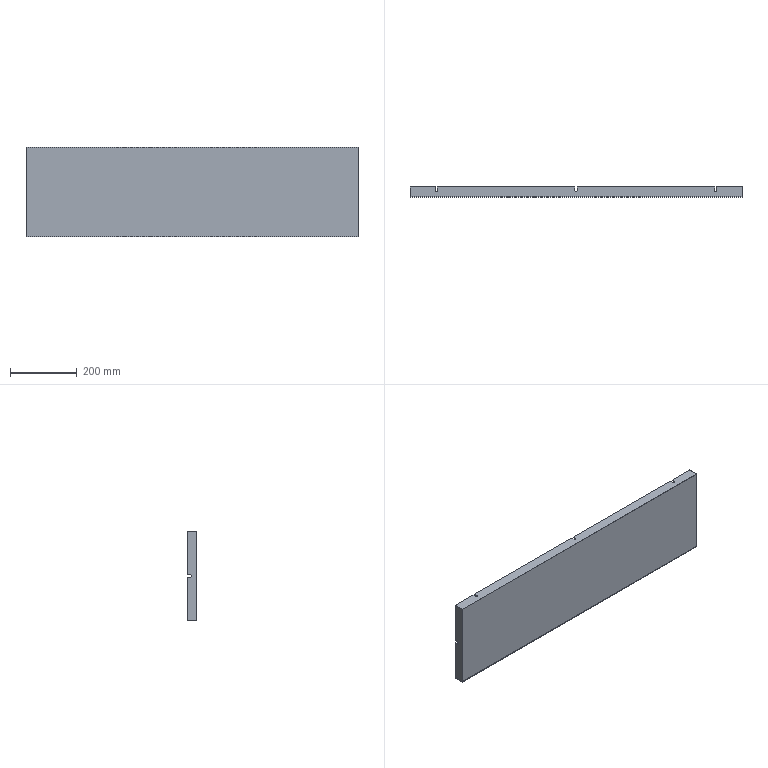Part | SolidWorks | features BaseBody 1 | 1 solid | 42 faces | box 998 x 30 x 268 mm | volume 508112 mm3 | plane 34 | cylinder 8 | commonest cylinder face diameters 7 x8
STEP:
#1=CARTESIAN_POINT('',(-416.5,20.,-132.5));
#2=VERTEX_POINT('',#1);
#3=CARTESIAN_POINT('',(-416.5,30.,-132.5));
#4=VERTEX_POINT('',#3);
#5=CARTESIAN_POINT('',(-416.5,30.,-132.5));
#6=DIRECTION('',(0.,1.,0.));
#7=VECTOR('',#6,1000.);
#8=LINE('',#5,#7);
#9=EDGE_CURVE('',#2,#4,#8,.T.);
#10=ORIENTED_EDGE('',*,*,#9,.T.);
#11=CARTESIAN_POINT('',(-416.5,30.,-134.));
#12=VERTEX_POINT('',#11);
#13=CARTESIAN_POINT('',(-416.5,30.,134.));
#14=DIRECTION('',(0.,0.,-1.));
#15=VECTOR('',#14,1000.);
#16=LINE('',#13,#15);
#17=EDGE_CURVE('',#4,#12,#16,.T.);
#18=ORIENTED_EDGE('',*,*,#17,.T.);
#19=CARTESIAN_POINT('',(-416.5,20.,-134.));
#20=VERTEX_POINT('',#19);
#21=CARTESIAN_POINT('',(-416.5,30.,-134.));
#22=DIRECTION('',(0.,-1.,0.));
#23=VECTOR('',#22,1000.);
#24=LINE('',#21,#23);
#25=EDGE_CURVE('',#12,#20,#24,.T.);
#26=ORIENTED_EDGE('',*,*,#25,.T.);
#27=CARTESIAN_POINT('',(-416.5,20.,134.));
#28=DIRECTION('',(0.,0.,-1.));
#29=VECTOR('',#28,1000.);
#30=LINE('',#27,#29);
#31=EDGE_CURVE('',#2,#20,#30,.T.);
#32=ORIENTED_EDGE('',*,*,#31,.F.);
#33=EDGE_LOOP('',(#10,#18,#26,#32));
#34=FACE_OUTER_BOUND('',#33,.T.);
#35=CARTESIAN_POINT('',(-416.5,30.,134.));
#36=DIRECTION('',(1.,0.,0.));
#37=DIRECTION('',(0.,1.,0.));
#38=AXIS2_PLACEMENT_3D('',#35,#36,#37);
#39=PLANE('',#38);
#40=ADVANCED_FACE('',(#34),#39,.F.);
#41=CARTESIAN_POINT('',(-423.5,20.,-132.5));
#42=VERTEX_POINT('',#41);
#43=CARTESIAN_POINT('',(-420.,20.,-132.5));
#44=DIRECTION('',(0.,0.,1.));
#45=DIRECTION('',(1.,0.,0.));
#46=AXIS2_PLACEMENT_3D('',#43,#44,#45);
#47=CIRCLE('',#46,3.5);
#48=EDGE_CURVE('',#42,#2,#47,.T.);
#49=ORIENTED_EDGE('',*,*,#48,.T.);
#50=ORIENTED_EDGE('',*,*,#31,.T.);
#51=CARTESIAN_POINT('',(-423.5,20.,-134.));
#52=VERTEX_POINT('',#51);
#53=CARTESIAN_POINT('',(-420.,20.,-134.));
#54=DIRECTION('',(0.,0.,-1.));
#55=DIRECTION('',(-1.,0.,0.));
#56=AXIS2_PLACEMENT_3D('',#53,#54,#55);
#57=CIRCLE('',#56,3.5);
#58=EDGE_CURVE('',#20,#52,#57,.T.);
#59=ORIENTED_EDGE('',*,*,#58,.T.);
#60=CARTESIAN_POINT('',(-423.5,20.,134.));
#61=DIRECTION('',(0.,0.,-1.));
#62=VECTOR('',#61,1000.);
#63=LINE('',#60,#62);
#64=EDGE_CURVE('',#42,#52,#63,.T.);
#65=ORIENTED_EDGE('',*,*,#64,.F.);
#66=EDGE_LOOP('',(#49,#50,#59,#65));
#67=FACE_OUTER_BOUND('',#66,.T.);
#68=CARTESIAN_POINT('',(-420.,20.,134.));
#69=DIRECTION('',(0.,0.,-1.));
#70=DIRECTION('',(-1.,0.,0.));
#71=AXIS2_PLACEMENT_3D('',#68,#69,#70);
#72=CYLINDRICAL_SURFACE('',#71,3.5);
#73=ADVANCED_FACE('',(#67),#72,.F.);
#74=CARTESIAN_POINT('',(-423.5,30.,-132.5));
#75=VERTEX_POINT('',#74);
#76=CARTESIAN_POINT('',(-423.5,30.,-132.5));
#77=DIRECTION('',(0.,-1.,0.));
#78=VECTOR('',#77,1000.);
#79=LINE('',#76,#78);
#80=EDGE_CURVE('',#75,#42,#79,.T.);
#81=ORIENTED_EDGE('',*,*,#80,.T.);
#82=ORIENTED_EDGE('',*,*,#64,.T.);
#83=CARTESIAN_POINT('',(-423.5,30.,-134.));
#84=VERTEX_POINT('',#83);
#85=CARTESIAN_POINT('',(-423.5,30.,-134.));
#86=DIRECTION('',(0.,1.,0.));
#87=VECTOR('',#86,1000.);
#88=LINE('',#85,#87);
#89=EDGE_CURVE('',#52,#84,#88,.T.);
#90=ORIENTED_EDGE('',*,*,#89,.T.);
#91=CARTESIAN_POINT('',(-423.5,30.,134.));
#92=DIRECTION('',(0.,0.,-1.));
#93=VECTOR('',#92,1000.);
#94=LINE('',#91,#93);
#95=EDGE_CURVE('',#75,#84,#94,.T.);
#96=ORIENTED_EDGE('',*,*,#95,.F.);
#97=EDGE_LOOP('',(#81,#82,#90,#96));
#98=FACE_OUTER_BOUND('',#97,.T.);
#99=CARTESIAN_POINT('',(-423.5,30.,134.));
#100=DIRECTION('',(-1.,0.,0.));
#101=DIRECTION('',(0.,0.,1.));
#102=AXIS2_PLACEMENT_3D('',#99,#100,#101);
#103=PLANE('',#102);
#104=ADVANCED_FACE('',(#98),#103,.F.);
#105=CARTESIAN_POINT('',(-423.5,20.,132.5));
#106=VERTEX_POINT('',#105);
#107=CARTESIAN_POINT('',(-423.5,30.,132.5));
#108=VERTEX_POINT('',#107);
#109=CARTESIAN_POINT('',(-423.5,30.,132.5));
#110=DIRECTION('',(0.,1.,0.));
#111=VECTOR('',#110,1000.);
#112=LINE('',#109,#111);
#113=EDGE_CURVE('',#106,#108,#112,.T.);
#114=ORIENTED_EDGE('',*,*,#113,.T.);
#115=CARTESIAN_POINT('',(-423.5,30.,134.));
#116=VERTEX_POINT('',#115);
#117=CARTESIAN_POINT('',(-423.5,30.,134.));
#118=DIRECTION('',(0.,0.,-1.));
#119=VECTOR('',#118,1000.);
#120=LINE('',#117,#119);
#121=EDGE_CURVE('',#116,#108,#120,.T.);
#122=ORIENTED_EDGE('',*,*,#121,.F.);
#123=CARTESIAN_POINT('',(-423.5,20.,134.));
#124=VERTEX_POINT('',#123);
#125=CARTESIAN_POINT('',(-423.5,30.,134.));
#126=DIRECTION('',(0.,1.,0.));
#127=VECTOR('',#126,1000.);
#128=LINE('',#125,#127);
#129=EDGE_CURVE('',#124,#116,#128,.T.);
#130=ORIENTED_EDGE('',*,*,#129,.F.);
#131=CARTESIAN_POINT('',(-423.5,20.,134.));
#132=DIRECTION('',(0.,0.,-1.));
#133=VECTOR('',#132,1000.);
#134=LINE('',#131,#133);
#135=EDGE_CURVE('',#124,#106,#134,.T.);
#136=ORIENTED_EDGE('',*,*,#135,.T.);
#137=EDGE_LOOP('',(#114,#122,#130,#136));
#138=FACE_OUTER_BOUND('',#137,.T.);
#139=CARTESIAN_POINT('',(-423.5,30.,134.));
#140=DIRECTION('',(-1.,0.,0.));
#141=DIRECTION('',(0.,0.,1.));
#142=AXIS2_PLACEMENT_3D('',#139,#140,#141);
#143=PLANE('',#142);
#144=ADVANCED_FACE('',(#138),#143,.F.);
#145=CARTESIAN_POINT('',(-416.5,20.,132.5));
#146=VERTEX_POINT('',#145);
#147=CARTESIAN_POINT('',(-420.,20.,132.5));
#148=DIRECTION('',(0.,0.,-1.));
#149=DIRECTION('',(-1.,0.,0.));
#150=AXIS2_PLACEMENT_3D('',#147,#148,#149);
#151=CIRCLE('',#150,3.5);
#152=EDGE_CURVE('',#146,#106,#151,.T.);
#153=ORIENTED_EDGE('',*,*,#152,.T.);
#154=ORIENTED_EDGE('',*,*,#135,.F.);
#155=CARTESIAN_POINT('',(-416.5,20.,134.));
#156=VERTEX_POINT('',#155);
#157=CARTESIAN_POINT('',(-420.,20.,134.));
#158=DIRECTION('',(0.,0.,-1.));
#159=DIRECTION('',(-1.,0.,0.));
#160=AXIS2_PLACEMENT_3D('',#157,#158,#159);
#161=CIRCLE('',#160,3.5);
#162=EDGE_CURVE('',#156,#124,#161,.T.);
#163=ORIENTED_EDGE('',*,*,#162,.F.);
#164=CARTESIAN_POINT('',(-416.5,20.,134.));
#165=DIRECTION('',(0.,0.,-1.));
#166=VECTOR('',#165,1000.);
#167=LINE('',#164,#166);
#168=EDGE_CURVE('',#156,#146,#167,.T.);
#169=ORIENTED_EDGE('',*,*,#168,.T.);
#170=EDGE_LOOP('',(#153,#154,#163,#169));
#171=FACE_OUTER_BOUND('',#170,.T.);
#172=CARTESIAN_POINT('',(-420.,20.,134.));
#173=DIRECTION('',(0.,0.,-1.));
#174=DIRECTION('',(-1.,0.,0.));
#175=AXIS2_PLACEMENT_3D('',#172,#173,#174);
#176=CYLINDRICAL_SURFACE('',#175,3.5);
#177=ADVANCED_FACE('',(#171),#176,.F.);
#178=CARTESIAN_POINT('',(-416.5,30.,132.5));
#179=VERTEX_POINT('',#178);
#180=CARTESIAN_POINT('',(-416.5,30.,132.5));
#181=DIRECTION('',(0.,-1.,0.));
#182=VECTOR('',#181,1000.);
#183=LINE('',#180,#182);
#184=EDGE_CURVE('',#179,#146,#183,.T.);
#185=ORIENTED_EDGE('',*,*,#184,.T.);
#186=ORIENTED_EDGE('',*,*,#168,.F.);
#187=CARTESIAN_POINT('',(-416.5,30.,134.));
#188=VERTEX_POINT('',#187);
#189=CARTESIAN_POINT('',(-416.5,30.,134.));
#190=DIRECTION('',(0.,-1.,0.));
#191=VECTOR('',#190,1000.);
#192=LINE('',#189,#191);
#193=EDGE_CURVE('',#188,#156,#192,.T.);
#194=ORIENTED_EDGE('',*,*,#193,.F.);
#195=CARTESIAN_POINT('',(-416.5,30.,134.));
#196=DIRECTION('',(0.,0.,-1.));
#197=VECTOR('',#196,1000.);
#198=LINE('',#195,#197);
#199=EDGE_CURVE('',#188,#179,#198,.T.);
#200=ORIENTED_EDGE('',*,*,#199,.T.);
#201=EDGE_LOOP('',(#185,#186,#194,#200));
#202=FACE_OUTER_BOUND('',#201,.T.);
#203=CARTESIAN_POINT('',(-416.5,30.,134.));
#204=DIRECTION('',(1.,0.,0.));
#205=DIRECTION('',(0.,1.,0.));
#206=AXIS2_PLACEMENT_3D('',#203,#204,#205);
#207=PLANE('',#206);
#208=ADVANCED_FACE('',(#202),#207,.F.);
#209=CARTESIAN_POINT('',(3.5,20.,-132.5));
#210=VERTEX_POINT('',#209);
#211=CARTESIAN_POINT('',(3.5,30.,-132.5));
#212=VERTEX_POINT('',#211);
#213=CARTESIAN_POINT('',(3.5,30.,-132.5));
#214=DIRECTION('',(0.,1.,0.));
#215=VECTOR('',#214,1000.);
#216=LINE('',#213,#215);
#217=EDGE_CURVE('',#210,#212,#216,.T.);
#218=ORIENTED_EDGE('',*,*,#217,.T.);
#219=CARTESIAN_POINT('',(3.5,30.,-134.));
#220=VERTEX_POINT('',#219);
#221=CARTESIAN_POINT('',(3.5,30.,134.));
#222=DIRECTION('',(0.,0.,-1.));
#223=VECTOR('',#222,1000.);
#224=LINE('',#221,#223);
#225=EDGE_CURVE('',#212,#220,#224,.T.);
#226=ORIENTED_EDGE('',*,*,#225,.T.);
#227=CARTESIAN_POINT('',(3.5,20.,-134.));
#228=VERTEX_POINT('',#227);
#229=CARTESIAN_POINT('',(3.5,30.,-134.));
#230=DIRECTION('',(0.,-1.,0.));
#231=VECTOR('',#230,1000.);
#232=LINE('',#229,#231);
#233=EDGE_CURVE('',#220,#228,#232,.T.);
#234=ORIENTED_EDGE('',*,*,#233,.T.);
#235=CARTESIAN_POINT('',(3.5,20.,134.));
#236=DIRECTION('',(0.,0.,-1.));
#237=VECTOR('',#236,1000.);
#238=LINE('',#235,#237);
#239=EDGE_CURVE('',#210,#228,#238,.T.);
#240=ORIENTED_EDGE('',*,*,#239,.F.);
#241=EDGE_LOOP('',(#218,#226,#234,#240));
#242=FACE_OUTER_BOUND('',#241,.T.);
#243=CARTESIAN_POINT('',(3.5,30.,134.));
#244=DIRECTION('',(1.,0.,0.));
#245=DIRECTION('',(0.,1.,0.));
#246=AXIS2_PLACEMENT_3D('',#243,#244,#245);
#247=PLANE('',#246);
#248=ADVANCED_FACE('',(#242),#247,.F.);
#249=CARTESIAN_POINT('',(-3.5,20.,-132.5));
#250=VERTEX_POINT('',#249);
#251=CARTESIAN_POINT('',(0.,20.,-132.5));
#252=DIRECTION('',(0.,0.,1.));
#253=DIRECTION('',(1.,0.,0.));
#254=AXIS2_PLACEMENT_3D('',#251,#252,#253);
#255=CIRCLE('',#254,3.5);
#256=EDGE_CURVE('',#250,#210,#255,.T.);
#257=ORIENTED_EDGE('',*,*,#256,.T.);
#258=ORIENTED_EDGE('',*,*,#239,.T.);
#259=CARTESIAN_POINT('',(-3.5,20.,-134.));
#260=VERTEX_POINT('',#259);
#261=CARTESIAN_POINT('',(0.,20.,-134.));
#262=DIRECTION('',(0.,0.,-1.));
#263=DIRECTION('',(-1.,0.,0.));
#264=AXIS2_PLACEMENT_3D('',#261,#262,#263);
#265=CIRCLE('',#264,3.5);
#266=EDGE_CURVE('',#228,#260,#265,.T.);
#267=ORIENTED_EDGE('',*,*,#266,.T.);
#268=CARTESIAN_POINT('',(-3.5,20.,134.));
#269=DIRECTION('',(0.,0.,-1.));
#270=VECTOR('',#269,1000.);
#271=LINE('',#268,#270);
#272=EDGE_CURVE('',#250,#260,#271,.T.);
#273=ORIENTED_EDGE('',*,*,#272,.F.);
#274=EDGE_LOOP('',(#257,#258,#267,#273));
#275=FACE_OUTER_BOUND('',#274,.T.);
#276=CARTESIAN_POINT('',(0.,20.,134.));
#277=DIRECTION('',(0.,0.,-1.));
#278=DIRECTION('',(-1.,0.,0.));
#279=AXIS2_PLACEMENT_3D('',#276,#277,#278);
#280=CYLINDRICAL_SURFACE('',#279,3.5);
#281=ADVANCED_FACE('',(#275),#280,.F.);
#282=CARTESIAN_POINT('',(-3.5,30.,-132.5));
#283=VERTEX_POINT('',#282);
#284=CARTESIAN_POINT('',(-3.5,30.,-132.5));
#285=DIRECTION('',(0.,-1.,0.));
#286=VECTOR('',#285,1000.);
#287=LINE('',#284,#286);
#288=EDGE_CURVE('',#283,#250,#287,.T.);
#289=ORIENTED_EDGE('',*,*,#288,.T.);
#290=ORIENTED_EDGE('',*,*,#272,.T.);
#291=CARTESIAN_POINT('',(-3.5,30.,-134.));
#292=VERTEX_POINT('',#291);
#293=CARTESIAN_POINT('',(-3.5,30.,-134.));
#294=DIRECTION('',(0.,1.,0.));
#295=VECTOR('',#294,1000.);
#296=LINE('',#293,#295);
#297=EDGE_CURVE('',#260,#292,#296,.T.);
#298=ORIENTED_EDGE('',*,*,#297,.T.);
#299=CARTESIAN_POINT('',(-3.5,30.,134.));
#300=DIRECTION('',(0.,0.,-1.));
#301=VECTOR('',#300,1000.);
#302=LINE('',#299,#301);
#303=EDGE_CURVE('',#283,#292,#302,.T.);
#304=ORIENTED_EDGE('',*,*,#303,.F.);
#305=EDGE_LOOP('',(#289,#290,#298,#304));
#306=FACE_OUTER_BOUND('',#305,.T.);
#307=CARTESIAN_POINT('',(-3.5,30.,134.));
#308=DIRECTION('',(-1.,0.,0.));
#309=DIRECTION('',(0.,0.,1.));
#310=AXIS2_PLACEMENT_3D('',#307,#308,#309);
#311=PLANE('',#310);
#312=ADVANCED_FACE('',(#306),#311,.F.);
#313=CARTESIAN_POINT('',(-3.5,20.,132.5));
#314=VERTEX_POINT('',#313);
#315=CARTESIAN_POINT('',(-3.5,30.,132.5));
#316=VERTEX_POINT('',#315);
#317=CARTESIAN_POINT('',(-3.5,30.,132.5));
#318=DIRECTION('',(0.,1.,0.));
#319=VECTOR('',#318,1000.);
#320=LINE('',#317,#319);
#321=EDGE_CURVE('',#314,#316,#320,.T.);
#322=ORIENTED_EDGE('',*,*,#321,.T.);
#323=CARTESIAN_POINT('',(-3.5,30.,134.));
#324=VERTEX_POINT('',#323);
#325=CARTESIAN_POINT('',(-3.5,30.,134.));
#326=DIRECTION('',(0.,0.,-1.));
#327=VECTOR('',#326,1000.);
#328=LINE('',#325,#327);
#329=EDGE_CURVE('',#324,#316,#328,.T.);
#330=ORIENTED_EDGE('',*,*,#329,.F.);
#331=CARTESIAN_POINT('',(-3.5,20.,134.));
#332=VERTEX_POINT('',#331);
#333=CARTESIAN_POINT('',(-3.5,30.,134.));
#334=DIRECTION('',(0.,1.,0.));
#335=VECTOR('',#334,1000.);
#336=LINE('',#333,#335);
#337=EDGE_CURVE('',#332,#324,#336,.T.);
#338=ORIENTED_EDGE('',*,*,#337,.F.);
#339=CARTESIAN_POINT('',(-3.5,20.,134.));
#340=DIRECTION('',(0.,0.,-1.));
#341=VECTOR('',#340,1000.);
#342=LINE('',#339,#341);
#343=EDGE_CURVE('',#332,#314,#342,.T.);
#344=ORIENTED_EDGE('',*,*,#343,.T.);
#345=EDGE_LOOP('',(#322,#330,#338,#344));
#346=FACE_OUTER_BOUND('',#345,.T.);
#347=CARTESIAN_POINT('',(-3.5,30.,134.));
#348=DIRECTION('',(-1.,0.,0.));
#349=DIRECTION('',(0.,0.,1.));
#350=AXIS2_PLACEMENT_3D('',#347,#348,#349);
#351=PLANE('',#350);
#352=ADVANCED_FACE('',(#346),#351,.F.);
#353=CARTESIAN_POINT('',(3.5,20.,132.5));
#354=VERTEX_POINT('',#353);
#355=CARTESIAN_POINT('',(0.,20.,132.5));
#356=DIRECTION('',(0.,0.,-1.));
#357=DIRECTION('',(-1.,0.,0.));
#358=AXIS2_PLACEMENT_3D('',#355,#356,#357);
#359=CIRCLE('',#358,3.5);
#360=EDGE_CURVE('',#354,#314,#359,.T.);
#361=ORIENTED_EDGE('',*,*,#360,.T.);
#362=ORIENTED_EDGE('',*,*,#343,.F.);
#363=CARTESIAN_POINT('',(3.5,20.,134.));
#364=VERTEX_POINT('',#363);
#365=CARTESIAN_POINT('',(0.,20.,134.));
#366=DIRECTION('',(0.,0.,-1.));
#367=DIRECTION('',(-1.,0.,0.));
#368=AXIS2_PLACEMENT_3D('',#365,#366,#367);
#369=CIRCLE('',#368,3.5);
#370=EDGE_CURVE('',#364,#332,#369,.T.);
#371=ORIENTED_EDGE('',*,*,#370,.F.);
#372=CARTESIAN_POINT('',(3.5,20.,134.));
#373=DIRECTION('',(0.,0.,-1.));
#374=VECTOR('',#373,1000.);
#375=LINE('',#372,#374);
#376=EDGE_CURVE('',#364,#354,#375,.T.);
#377=ORIENTED_EDGE('',*,*,#376,.T.);
#378=EDGE_LOOP('',(#361,#362,#371,#377));
#379=FACE_OUTER_BOUND('',#378,.T.);
#380=CARTESIAN_POINT('',(0.,20.,134.));
#381=DIRECTION('',(0.,0.,-1.));
#382=DIRECTION('',(-1.,0.,0.));
#383=AXIS2_PLACEMENT_3D('',#380,#381,#382);
#384=CYLINDRICAL_SURFACE('',#383,3.5);
#385=ADVANCED_FACE('',(#379),#384,.F.);
#386=CARTESIAN_POINT('',(3.5,30.,132.5));
#387=VERTEX_POINT('',#386);
#388=CARTESIAN_POINT('',(3.5,30.,132.5));
#389=DIRECTION('',(0.,-1.,0.));
#390=VECTOR('',#389,1000.);
#391=LINE('',#388,#390);
#392=EDGE_CURVE('',#387,#354,#391,.T.);
#393=ORIENTED_EDGE('',*,*,#392,.T.);
#394=ORIENTED_EDGE('',*,*,#376,.F.);
#395=CARTESIAN_POINT('',(3.5,30.,134.));
#396=VERTEX_POINT('',#395);
#397=CARTESIAN_POINT('',(3.5,30.,134.));
#398=DIRECTION('',(0.,-1.,0.));
#399=VECTOR('',#398,1000.);
#400=LINE('',#397,#399);
#401=EDGE_CURVE('',#396,#364,#400,.T.);
#402=ORIENTED_EDGE('',*,*,#401,.F.);
#403=CARTESIAN_POINT('',(3.5,30.,134.));
#404=DIRECTION('',(0.,0.,-1.));
#405=VECTOR('',#404,1000.);
#406=LINE('',#403,#405);
#407=EDGE_CURVE('',#396,#387,#406,.T.);
#408=ORIENTED_EDGE('',*,*,#407,.T.);
#409=EDGE_LOOP('',(#393,#394,#402,#408));
#410=FACE_OUTER_BOUND('',#409,.T.);
#411=CARTESIAN_POINT('',(3.5,30.,134.));
#412=DIRECTION('',(1.,0.,0.));
#413=DIRECTION('',(0.,1.,0.));
#414=AXIS2_PLACEMENT_3D('',#411,#412,#413);
#415=PLANE('',#414);
#416=ADVANCED_FACE('',(#410),#415,.F.);
#417=CARTESIAN_POINT('',(423.5,20.,-132.5));
#418=VERTEX_POINT('',#417);
#419=CARTESIAN_POINT('',(423.5,30.,-132.5));
#420=VERTEX_POINT('',#419);
#421=CARTESIAN_POINT('',(423.5,30.,-132.5));
#422=DIRECTION('',(0.,1.,0.));
#423=VECTOR('',#422,1000.);
#424=LINE('',#421,#423);
#425=EDGE_CURVE('',#418,#420,#424,.T.);
#426=ORIENTED_EDGE('',*,*,#425,.T.);
#427=CARTESIAN_POINT('',(423.5,30.,-134.));
#428=VERTEX_POINT('',#427);
#429=CARTESIAN_POINT('',(423.5,30.,134.));
#430=DIRECTION('',(0.,0.,-1.));
#431=VECTOR('',#430,1000.);
#432=LINE('',#429,#431);
#433=EDGE_CURVE('',#420,#428,#432,.T.);
#434=ORIENTED_EDGE('',*,*,#433,.T.);
#435=CARTESIAN_POINT('',(423.5,20.,-134.));
#436=VERTEX_POINT('',#435);
#437=CARTESIAN_POINT('',(423.5,30.,-134.));
#438=DIRECTION('',(0.,-1.,0.));
#439=VECTOR('',#438,1000.);
#440=LINE('',#437,#439);
#441=EDGE_CURVE('',#428,#436,#440,.T.);
#442=ORIENTED_EDGE('',*,*,#441,.T.);
#443=CARTESIAN_POINT('',(423.5,20.,134.));
#444=DIRECTION('',(0.,0.,-1.));
#445=VECTOR('',#444,1000.);
#446=LINE('',#443,#445);
#447=EDGE_CURVE('',#418,#436,#446,.T.);
#448=ORIENTED_EDGE('',*,*,#447,.F.);
#449=EDGE_LOOP('',(#426,#434,#442,#448));
#450=FACE_OUTER_BOUND('',#449,.T.);
#451=CARTESIAN_POINT('',(423.5,30.,134.));
#452=DIRECTION('',(1.,0.,0.));
#453=DIRECTION('',(0.,1.,0.));
#454=AXIS2_PLACEMENT_3D('',#451,#452,#453);
#455=PLANE('',#454);
#456=ADVANCED_FACE('',(#450),#455,.F.);
#457=CARTESIAN_POINT('',(416.5,20.,-132.5));
#458=VERTEX_POINT('',#457);
#459=CARTESIAN_POINT('',(420.,20.,-132.5));
#460=DIRECTION('',(0.,0.,1.));
#461=DIRECTION('',(1.,0.,0.));
#462=AXIS2_PLACEMENT_3D('',#459,#460,#461);
#463=CIRCLE('',#462,3.5);
#464=EDGE_CURVE('',#458,#418,#463,.T.);
#465=ORIENTED_EDGE('',*,*,#464,.T.);
#466=ORIENTED_EDGE('',*,*,#447,.T.);
#467=CARTESIAN_POINT('',(416.5,20.,-134.));
#468=VERTEX_POINT('',#467);
#469=CARTESIAN_POINT('',(420.,20.,-134.));
#470=DIRECTION('',(0.,0.,-1.));
#471=DIRECTION('',(-1.,0.,0.));
#472=AXIS2_PLACEMENT_3D('',#469,#470,#471);
#473=CIRCLE('',#472,3.5);
#474=EDGE_CURVE('',#436,#468,#473,.T.);
#475=ORIENTED_EDGE('',*,*,#474,.T.);
#476=CARTESIAN_POINT('',(416.5,20.,134.));
#477=DIRECTION('',(0.,0.,-1.));
#478=VECTOR('',#477,1000.);
#479=LINE('',#476,#478);
#480=EDGE_CURVE('',#458,#468,#479,.T.);
#481=ORIENTED_EDGE('',*,*,#480,.F.);
#482=EDGE_LOOP('',(#465,#466,#475,#481));
#483=FACE_OUTER_BOUND('',#482,.T.);
#484=CARTESIAN_POINT('',(420.,20.,134.));
#485=DIRECTION('',(0.,0.,-1.));
#486=DIRECTION('',(-1.,0.,0.));
#487=AXIS2_PLACEMENT_3D('',#484,#485,#486);
#488=CYLINDRICAL_SURFACE('',#487,3.5);
#489=ADVANCED_FACE('',(#483),#488,.F.);
#490=CARTESIAN_POINT('',(416.5,30.,-132.5));
#491=VERTEX_POINT('',#490);
#492=CARTESIAN_POINT('',(416.5,30.,-132.5));
#493=DIRECTION('',(0.,-1.,0.));
#494=VECTOR('',#493,1000.);
#495=LINE('',#492,#494);
#496=EDGE_CURVE('',#491,#458,#495,.T.);
#497=ORIENTED_EDGE('',*,*,#496,.T.);
#498=ORIENTED_EDGE('',*,*,#480,.T.);
#499=CARTESIAN_POINT('',(416.5,30.,-134.));
#500=VERTEX_POINT('',#499);
#501=CARTESIAN_POINT('',(416.5,30.,-134.));
#502=DIRECTION('',(0.,1.,0.));
#503=VECTOR('',#502,1000.);
#504=LINE('',#501,#503);
#505=EDGE_CURVE('',#468,#500,#504,.T.);
#506=ORIENTED_EDGE('',*,*,#505,.T.);
#507=CARTESIAN_POINT('',(416.5,30.,134.));
#508=DIRECTION('',(0.,0.,-1.));
#509=VECTOR('',#508,1000.);
#510=LINE('',#507,#509);
#511=EDGE_CURVE('',#491,#500,#510,.T.);
#512=ORIENTED_EDGE('',*,*,#511,.F.);
#513=EDGE_LOOP('',(#497,#498,#506,#512));
#514=FACE_OUTER_BOUND('',#513,.T.);
#515=CARTESIAN_POINT('',(416.5,30.,134.));
#516=DIRECTION('',(-1.,0.,0.));
#517=DIRECTION('',(0.,0.,1.));
#518=AXIS2_PLACEMENT_3D('',#515,#516,#517);
#519=PLANE('',#518);
#520=ADVANCED_FACE('',(#514),#519,.F.);
#521=CARTESIAN_POINT('',(416.5,20.,132.5));
#522=VERTEX_POINT('',#521);
#523=CARTESIAN_POINT('',(416.5,30.,132.5));
#524=VERTEX_POINT('',#523);
#525=CARTESIAN_POINT('',(416.5,30.,132.5));
#526=DIRECTION('',(0.,1.,0.));
#527=VECTOR('',#526,1000.);
#528=LINE('',#525,#527);
#529=EDGE_CURVE('',#522,#524,#528,.T.);
#530=ORIENTED_EDGE('',*,*,#529,.T.);
#531=CARTESIAN_POINT('',(416.5,30.,134.));
#532=VERTEX_POINT('',#531);
#533=CARTESIAN_POINT('',(416.5,30.,134.));
#534=DIRECTION('',(0.,0.,-1.));
#535=VECTOR('',#534,1000.);
#536=LINE('',#533,#535);
#537=EDGE_CURVE('',#532,#524,#536,.T.);
#538=ORIENTED_EDGE('',*,*,#537,.F.);
#539=CARTESIAN_POINT('',(416.5,20.,134.));
#540=VERTEX_POINT('',#539);
#541=CARTESIAN_POINT('',(416.5,30.,134.));
#542=DIRECTION('',(0.,1.,0.));
#543=VECTOR('',#542,1000.);
#544=LINE('',#541,#543);
#545=EDGE_CURVE('',#540,#532,#544,.T.);
#546=ORIENTED_EDGE('',*,*,#545,.F.);
#547=CARTESIAN_POINT('',(416.5,20.,134.));
#548=DIRECTION('',(0.,0.,-1.));
#549=VECTOR('',#548,1000.);
#550=LINE('',#547,#549);
#551=EDGE_CURVE('',#540,#522,#550,.T.);
#552=ORIENTED_EDGE('',*,*,#551,.T.);
#553=EDGE_LOOP('',(#530,#538,#546,#552));
#554=FACE_OUTER_BOUND('',#553,.T.);
#555=CARTESIAN_POINT('',(416.5,30.,134.));
#556=DIRECTION('',(-1.,0.,0.));
#557=DIRECTION('',(0.,0.,1.));
#558=AXIS2_PLACEMENT_3D('',#555,#556,#557);
#559=PLANE('',#558);
#560=ADVANCED_FACE('',(#554),#559,.F.);
#561=CARTESIAN_POINT('',(423.5,20.,132.5));
#562=VERTEX_POINT('',#561);
#563=CARTESIAN_POINT('',(420.,20.,132.5));
#564=DIRECTION('',(0.,0.,-1.));
#565=DIRECTION('',(-1.,0.,0.));
#566=AXIS2_PLACEMENT_3D('',#563,#564,#565);
#567=CIRCLE('',#566,3.5);
#568=EDGE_CURVE('',#562,#522,#567,.T.);
#569=ORIENTED_EDGE('',*,*,#568,.T.);
#570=ORIENTED_EDGE('',*,*,#551,.F.);
#571=CARTESIAN_POINT('',(423.5,20.,134.));
#572=VERTEX_POINT('',#571);
#573=CARTESIAN_POINT('',(420.,20.,134.));
#574=DIRECTION('',(0.,0.,-1.));
#575=DIRECTION('',(-1.,0.,0.));
#576=AXIS2_PLACEMENT_3D('',#573,#574,#575);
#577=CIRCLE('',#576,3.5);
#578=EDGE_CURVE('',#572,#540,#577,.T.);
#579=ORIENTED_EDGE('',*,*,#578,.F.);
#580=CARTESIAN_POINT('',(423.5,20.,134.));
#581=DIRECTION('',(0.,0.,-1.));
#582=VECTOR('',#581,1000.);
#583=LINE('',#580,#582);
#584=EDGE_CURVE('',#572,#562,#583,.T.);
#585=ORIENTED_EDGE('',*,*,#584,.T.);
#586=EDGE_LOOP('',(#569,#570,#579,#585));
#587=FACE_OUTER_BOUND('',#586,.T.);
#588=CARTESIAN_POINT('',(420.,20.,134.));
#589=DIRECTION('',(0.,0.,-1.));
#590=DIRECTION('',(-1.,0.,0.));
#591=AXIS2_PLACEMENT_3D('',#588,#589,#590);
#592=CYLINDRICAL_SURFACE('',#591,3.5);
#593=ADVANCED_FACE('',(#587),#592,.F.);
#594=CARTESIAN_POINT('',(423.5,30.,132.5));
#595=VERTEX_POINT('',#594);
#596=CARTESIAN_POINT('',(423.5,30.,132.5));
#597=DIRECTION('',(0.,-1.,0.));
#598=VECTOR('',#597,1000.);
#599=LINE('',#596,#598);
#600=EDGE_CURVE('',#595,#562,#599,.T.);
#601=ORIENTED_EDGE('',*,*,#600,.T.);
#602=ORIENTED_EDGE('',*,*,#584,.F.);
#603=CARTESIAN_POINT('',(423.5,30.,134.));
#604=VERTEX_POINT('',#603);
#605=CARTESIAN_POINT('',(423.5,30.,134.));
#606=DIRECTION('',(0.,-1.,0.));
#607=VECTOR('',#606,1000.);
#608=LINE('',#605,#607);
#609=EDGE_CURVE('',#604,#572,#608,.T.);
#610=ORIENTED_EDGE('',*,*,#609,.F.);
#611=CARTESIAN_POINT('',(423.5,30.,134.));
#612=DIRECTION('',(0.,0.,-1.));
#613=VECTOR('',#612,1000.);
#614=LINE('',#611,#613);
#615=EDGE_CURVE('',#604,#595,#614,.T.);
#616=ORIENTED_EDGE('',*,*,#615,.T.);
#617=EDGE_LOOP('',(#601,#602,#610,#616));
#618=FACE_OUTER_BOUND('',#617,.T.);
#619=CARTESIAN_POINT('',(423.5,30.,134.));
#620=DIRECTION('',(1.,0.,0.));
#621=DIRECTION('',(0.,1.,0.));
#622=AXIS2_PLACEMENT_3D('',#619,#620,#621);
#623=PLANE('',#622);
#624=ADVANCED_FACE('',(#618),#623,.F.);
#625=CARTESIAN_POINT('',(497.5,20.,3.5));
#626=VERTEX_POINT('',#625);
#627=CARTESIAN_POINT('',(497.5,30.,3.5));
#628=VERTEX_POINT('',#627);
#629=CARTESIAN_POINT('',(497.5,30.,3.5));
#630=DIRECTION('',(0.,1.,0.));
#631=VECTOR('',#630,1000.);
#632=LINE('',#629,#631);
#633=EDGE_CURVE('',#626,#628,#632,.T.);
#634=ORIENTED_EDGE('',*,*,#633,.T.);
#635=CARTESIAN_POINT('',(499.,30.,3.5));
#636=VERTEX_POINT('',#635);
#637=CARTESIAN_POINT('',(-499.,30.,3.5));
#638=DIRECTION('',(1.,0.,0.));
#639=VECTOR('',#638,1000.);
#640=LINE('',#637,#639);
#641=EDGE_CURVE('',#628,#636,#640,.T.);
#642=ORIENTED_EDGE('',*,*,#641,.T.);
#643=CARTESIAN_POINT('',(499.,20.,3.5));
#644=VERTEX_POINT('',#643);
#645=CARTESIAN_POINT('',(499.,30.,3.5));
#646=DIRECTION('',(0.,-1.,0.));
#647=VECTOR('',#646,1000.);
#648=LINE('',#645,#647);
#649=EDGE_CURVE('',#636,#644,#648,.T.);
#650=ORIENTED_EDGE('',*,*,#649,.T.);
#651=CARTESIAN_POINT('',(-499.,20.,3.5));
#652=DIRECTION('',(1.,0.,0.));
#653=VECTOR('',#652,1000.);
#654=LINE('',#651,#653);
#655=EDGE_CURVE('',#626,#644,#654,.T.);
#656=ORIENTED_EDGE('',*,*,#655,.F.);
#657=EDGE_LOOP('',(#634,#642,#650,#656));
#658=FACE_OUTER_BOUND('',#657,.T.);
#659=CARTESIAN_POINT('',(-499.,30.,3.5));
#660=DIRECTION('',(0.,0.,1.));
#661=DIRECTION('',(0.,-1.,0.));
#662=AXIS2_PLACEMENT_3D('',#659,#660,#661);
#663=PLANE('',#662);
#664=ADVANCED_FACE('',(#658),#663,.F.);
#665=CARTESIAN_POINT('',(497.5,20.,-3.5));
#666=VERTEX_POINT('',#665);
#667=CARTESIAN_POINT('',(497.5,20.,0.));
#668=DIRECTION('',(-1.,0.,0.));
#669=DIRECTION('',(0.,0.,1.));
#670=AXIS2_PLACEMENT_3D('',#667,#668,#669);
#671=CIRCLE('',#670,3.5);
#672=EDGE_CURVE('',#666,#626,#671,.T.);
#673=ORIENTED_EDGE('',*,*,#672,.T.);
#674=ORIENTED_EDGE('',*,*,#655,.T.);
#675=CARTESIAN_POINT('',(499.,20.,-3.5));
#676=VERTEX_POINT('',#675);
#677=CARTESIAN_POINT('',(499.,20.,0.));
#678=DIRECTION('',(1.,0.,0.));
#679=DIRECTION('',(0.,0.,-1.));
#680=AXIS2_PLACEMENT_3D('',#677,#678,#679);
#681=CIRCLE('',#680,3.5);
#682=EDGE_CURVE('',#644,#676,#681,.T.);
#683=ORIENTED_EDGE('',*,*,#682,.T.);
#684=CARTESIAN_POINT('',(-499.,20.,-3.5));
#685=DIRECTION('',(1.,0.,0.));
#686=VECTOR('',#685,1000.);
#687=LINE('',#684,#686);
#688=EDGE_CURVE('',#666,#676,#687,.T.);
#689=ORIENTED_EDGE('',*,*,#688,.F.);
#690=EDGE_LOOP('',(#673,#674,#683,#689));
#691=FACE_OUTER_BOUND('',#690,.T.);
#692=CARTESIAN_POINT('',(-499.,20.,0.));
#693=DIRECTION('',(1.,0.,0.));
#694=DIRECTION('',(0.,0.,-1.));
#695=AXIS2_PLACEMENT_3D('',#692,#693,#694);
#696=CYLINDRICAL_SURFACE('',#695,3.5);
#697=ADVANCED_FACE('',(#691),#696,.F.);
#698=CARTESIAN_POINT('',(497.5,30.,-3.5));
#699=VERTEX_POINT('',#698);
#700=CARTESIAN_POINT('',(497.5,30.,-3.5));
#701=DIRECTION('',(0.,-1.,0.));
#702=VECTOR('',#701,1000.);
#703=LINE('',#700,#702);
#704=EDGE_CURVE('',#699,#666,#703,.T.);
#705=ORIENTED_EDGE('',*,*,#704,.T.);
#706=ORIENTED_EDGE('',*,*,#688,.T.);
#707=CARTESIAN_POINT('',(499.,30.,-3.5));
#708=VERTEX_POINT('',#707);
#709=CARTESIAN_POINT('',(499.,30.,-3.5));
#710=DIRECTION('',(0.,1.,0.));
#711=VECTOR('',#710,1000.);
#712=LINE('',#709,#711);
#713=EDGE_CURVE('',#676,#708,#712,.T.);
#714=ORIENTED_EDGE('',*,*,#713,.T.);
#715=CARTESIAN_POINT('',(-499.,30.,-3.5));
#716=DIRECTION('',(1.,0.,0.));
#717=VECTOR('',#716,1000.);
#718=LINE('',#715,#717);
#719=EDGE_CURVE('',#699,#708,#718,.T.);
#720=ORIENTED_EDGE('',*,*,#719,.F.);
#721=EDGE_LOOP('',(#705,#706,#714,#720));
#722=FACE_OUTER_BOUND('',#721,.T.);
#723=CARTESIAN_POINT('',(-499.,30.,-3.5));
#724=DIRECTION('',(0.,0.,-1.));
#725=DIRECTION('',(-1.,0.,0.));
#726=AXIS2_PLACEMENT_3D('',#723,#724,#725);
#727=PLANE('',#726);
#728=ADVANCED_FACE('',(#722),#727,.F.);
#729=CARTESIAN_POINT('',(-497.5,20.,-3.5));
#730=VERTEX_POINT('',#729);
#731=CARTESIAN_POINT('',(-497.5,30.,-3.5));
#732=VERTEX_POINT('',#731);
#733=CARTESIAN_POINT('',(-497.5,30.,-3.5));
#734=DIRECTION('',(0.,1.,0.));
#735=VECTOR('',#734,1000.);
#736=LINE('',#733,#735);
#737=EDGE_CURVE('',#730,#732,#736,.T.);
#738=ORIENTED_EDGE('',*,*,#737,.T.);
#739=CARTESIAN_POINT('',(-499.,30.,-3.5));
#740=VERTEX_POINT('',#739);
#741=CARTESIAN_POINT('',(-499.,30.,-3.5));
#742=DIRECTION('',(1.,0.,0.));
#743=VECTOR('',#742,1000.);
#744=LINE('',#741,#743);
#745=EDGE_CURVE('',#740,#732,#744,.T.);
#746=ORIENTED_EDGE('',*,*,#745,.F.);
#747=CARTESIAN_POINT('',(-499.,20.,-3.5));
#748=VERTEX_POINT('',#747);
#749=CARTESIAN_POINT('',(-499.,30.,-3.5));
#750=DIRECTION('',(0.,1.,0.));
#751=VECTOR('',#750,1000.);
#752=LINE('',#749,#751);
#753=EDGE_CURVE('',#748,#740,#752,.T.);
#754=ORIENTED_EDGE('',*,*,#753,.F.);
#755=CARTESIAN_POINT('',(-499.,20.,-3.5));
#756=DIRECTION('',(1.,0.,0.));
#757=VECTOR('',#756,1000.);
#758=LINE('',#755,#757);
#759=EDGE_CURVE('',#748,#730,#758,.T.);
#760=ORIENTED_EDGE('',*,*,#759,.T.);
#761=EDGE_LOOP('',(#738,#746,#754,#760));
#762=FACE_OUTER_BOUND('',#761,.T.);
#763=CARTESIAN_POINT('',(-499.,30.,-3.5));
#764=DIRECTION('',(0.,0.,-1.));
#765=DIRECTION('',(-1.,0.,0.));
#766=AXIS2_PLACEMENT_3D('',#763,#764,#765);
#767=PLANE('',#766);
#768=ADVANCED_FACE('',(#762),#767,.F.);
#769=CARTESIAN_POINT('',(-497.5,20.,3.5));
#770=VERTEX_POINT('',#769);
#771=CARTESIAN_POINT('',(-497.5,20.,0.));
#772=DIRECTION('',(1.,0.,0.));
#773=DIRECTION('',(0.,0.,-1.));
#774=AXIS2_PLACEMENT_3D('',#771,#772,#773);
#775=CIRCLE('',#774,3.5);
#776=EDGE_CURVE('',#770,#730,#775,.T.);
#777=ORIENTED_EDGE('',*,*,#776,.T.);
#778=ORIENTED_EDGE('',*,*,#759,.F.);
#779=CARTESIAN_POINT('',(-499.,20.,3.5));
#780=VERTEX_POINT('',#779);
#781=CARTESIAN_POINT('',(-499.,20.,0.));
#782=DIRECTION('',(1.,0.,0.));
#783=DIRECTION('',(0.,0.,-1.));
#784=AXIS2_PLACEMENT_3D('',#781,#782,#783);
#785=CIRCLE('',#784,3.5);
#786=EDGE_CURVE('',#780,#748,#785,.T.);
#787=ORIENTED_EDGE('',*,*,#786,.F.);
#788=CARTESIAN_POINT('',(-499.,20.,3.5));
#789=DIRECTION('',(1.,0.,0.));
#790=VECTOR('',#789,1000.);
#791=LINE('',#788,#790);
#792=EDGE_CURVE('',#780,#770,#791,.T.);
#793=ORIENTED_EDGE('',*,*,#792,.T.);
#794=EDGE_LOOP('',(#777,#778,#787,#793));
#795=FACE_OUTER_BOUND('',#794,.T.);
#796=CARTESIAN_POINT('',(-499.,20.,0.));
#797=DIRECTION('',(1.,0.,0.));
#798=DIRECTION('',(0.,0.,-1.));
#799=AXIS2_PLACEMENT_3D('',#796,#797,#798);
#800=CYLINDRICAL_SURFACE('',#799,3.5);
#801=ADVANCED_FACE('',(#795),#800,.F.);
#802=CARTESIAN_POINT('',(-497.5,30.,3.5));
#803=VERTEX_POINT('',#802);
#804=CARTESIAN_POINT('',(-497.5,30.,3.5));
#805=DIRECTION('',(0.,-1.,0.));
#806=VECTOR('',#805,1000.);
#807=LINE('',#804,#806);
#808=EDGE_CURVE('',#803,#770,#807,.T.);
#809=ORIENTED_EDGE('',*,*,#808,.T.);
#810=ORIENTED_EDGE('',*,*,#792,.F.);
#811=CARTESIAN_POINT('',(-499.,30.,3.5));
#812=VERTEX_POINT('',#811);
#813=CARTESIAN_POINT('',(-499.,30.,3.5));
#814=DIRECTION('',(0.,-1.,0.));
#815=VECTOR('',#814,1000.);
#816=LINE('',#813,#815);
#817=EDGE_CURVE('',#812,#780,#816,.T.);
#818=ORIENTED_EDGE('',*,*,#817,.F.);
#819=CARTESIAN_POINT('',(-499.,30.,3.5));
#820=DIRECTION('',(1.,0.,0.));
#821=VECTOR('',#820,1000.);
#822=LINE('',#819,#821);
#823=EDGE_CURVE('',#812,#803,#822,.T.);
#824=ORIENTED_EDGE('',*,*,#823,.T.);
#825=EDGE_LOOP('',(#809,#810,#818,#824));
#826=FACE_OUTER_BOUND('',#825,.T.);
#827=CARTESIAN_POINT('',(-499.,30.,3.5));
#828=DIRECTION('',(0.,0.,1.));
#829=DIRECTION('',(0.,-1.,0.));
#830=AXIS2_PLACEMENT_3D('',#827,#828,#829);
#831=PLANE('',#830);
#832=ADVANCED_FACE('',(#826),#831,.F.);
#833=CARTESIAN_POINT('',(497.5,1.5,132.5));
#834=VERTEX_POINT('',#833);
#835=CARTESIAN_POINT('',(497.5,1.5,-132.5));
#836=VERTEX_POINT('',#835);
#837=CARTESIAN_POINT('',(497.5,1.5,0.));
#838=DIRECTION('',(0.,0.,-1.));
#839=VECTOR('',#838,1000.);
#840=LINE('',#837,#839);
#841=EDGE_CURVE('',#834,#836,#840,.T.);
#842=ORIENTED_EDGE('',*,*,#841,.T.);
#843=CARTESIAN_POINT('',(-497.5,1.5,-132.5));
#844=VERTEX_POINT('',#843);
#845=CARTESIAN_POINT('',(0.,1.5,-132.5));
#846=DIRECTION('',(-1.,0.,0.));
#847=VECTOR('',#846,1000.);
#848=LINE('',#845,#847);
#849=EDGE_CURVE('',#836,#844,#848,.T.);
#850=ORIENTED_EDGE('',*,*,#849,.T.);
#851=CARTESIAN_POINT('',(-497.5,1.5,132.5));
#852=VERTEX_POINT('',#851);
#853=CARTESIAN_POINT('',(-497.5,1.5,0.));
#854=DIRECTION('',(0.,0.,1.));
#855=VECTOR('',#854,1000.);
#856=LINE('',#853,#855);
#857=EDGE_CURVE('',#844,#852,#856,.T.);
#858=ORIENTED_EDGE('',*,*,#857,.T.);
#859=CARTESIAN_POINT('',(0.,1.5,132.5));
#860=DIRECTION('',(1.,0.,0.));
#861=VECTOR('',#860,1000.);
#862=LINE('',#859,#861);
#863=EDGE_CURVE('',#852,#834,#862,.T.);
#864=ORIENTED_EDGE('',*,*,#863,.T.);
#865=EDGE_LOOP('',(#842,#850,#858,#864));
#866=FACE_OUTER_BOUND('',#865,.T.);
#867=CARTESIAN_POINT('',(0.,1.5,0.));
#868=DIRECTION('',(0.,-1.,0.));
#869=DIRECTION('',(0.,0.,-1.));
#870=AXIS2_PLACEMENT_3D('',#867,#868,#869);
#871=PLANE('',#870);
#872=ADVANCED_FACE('',(#866),#871,.F.);
#873=ORIENTED_EDGE('',*,*,#113,.F.);
#874=ORIENTED_EDGE('',*,*,#152,.F.);
#875=ORIENTED_EDGE('',*,*,#184,.F.);
#876=CARTESIAN_POINT('',(0.,30.,132.5));
#877=DIRECTION('',(1.,0.,0.));
#878=VECTOR('',#877,1000.);
#879=LINE('',#876,#878);
#880=EDGE_CURVE('',#179,#316,#879,.T.);
#881=ORIENTED_EDGE('',*,*,#880,.T.);
#882=ORIENTED_EDGE('',*,*,#321,.F.);
#883=ORIENTED_EDGE('',*,*,#360,.F.);
#884=ORIENTED_EDGE('',*,*,#392,.F.);
#885=CARTESIAN_POINT('',(0.,30.,132.5));
#886=DIRECTION('',(1.,0.,0.));
#887=VECTOR('',#886,1000.);
#888=LINE('',#885,#887);
#889=EDGE_CURVE('',#387,#524,#888,.T.);
#890=ORIENTED_EDGE('',*,*,#889,.T.);
#891=ORIENTED_EDGE('',*,*,#529,.F.);
#892=ORIENTED_EDGE('',*,*,#568,.F.);
#893=ORIENTED_EDGE('',*,*,#600,.F.);
#894=CARTESIAN_POINT('',(497.5,30.,132.5));
#895=VERTEX_POINT('',#894);
#896=CARTESIAN_POINT('',(0.,30.,132.5));
#897=DIRECTION('',(1.,0.,0.));
#898=VECTOR('',#897,1000.);
#899=LINE('',#896,#898);
#900=EDGE_CURVE('',#595,#895,#899,.T.);
#901=ORIENTED_EDGE('',*,*,#900,.T.);
#902=CARTESIAN_POINT('',(497.5,30.,132.5));
#903=DIRECTION('',(0.,-1.,0.));
#904=VECTOR('',#903,1000.);
#905=LINE('',#902,#904);
#906=EDGE_CURVE('',#895,#834,#905,.T.);
#907=ORIENTED_EDGE('',*,*,#906,.T.);
#908=ORIENTED_EDGE('',*,*,#863,.F.);
#909=CARTESIAN_POINT('',(-497.5,30.,132.5));
#910=VERTEX_POINT('',#909);
#911=CARTESIAN_POINT('',(-497.5,30.,132.5));
#912=DIRECTION('',(0.,-1.,0.));
#913=VECTOR('',#912,1000.);
#914=LINE('',#911,#913);
#915=EDGE_CURVE('',#910,#852,#914,.T.);
#916=ORIENTED_EDGE('',*,*,#915,.F.);
#917=CARTESIAN_POINT('',(0.,30.,132.5));
#918=DIRECTION('',(1.,0.,0.));
#919=VECTOR('',#918,1000.);
#920=LINE('',#917,#919);
#921=EDGE_CURVE('',#910,#108,#920,.T.);
#922=ORIENTED_EDGE('',*,*,#921,.T.);
#923=EDGE_LOOP('',(#873,#874,#875,#881,#882,#883,#884,#890,#891,#892,#893,#901,#907,#908,#916,#922));
#924=FACE_OUTER_BOUND('',#923,.T.);
#925=CARTESIAN_POINT('',(-499.,30.,132.5));
#926=DIRECTION('',(0.,0.,-1.));
#927=DIRECTION('',(0.,-1.,0.));
#928=AXIS2_PLACEMENT_3D('',#925,#926,#927);
#929=PLANE('',#928);
#930=ADVANCED_FACE('',(#924),#929,.T.);
#931=ORIENTED_EDGE('',*,*,#737,.F.);
#932=ORIENTED_EDGE('',*,*,#776,.F.);
#933=ORIENTED_EDGE('',*,*,#808,.F.);
#934=CARTESIAN_POINT('',(-497.5,30.,0.));
#935=DIRECTION('',(0.,0.,1.));
#936=VECTOR('',#935,1000.);
#937=LINE('',#934,#936);
#938=EDGE_CURVE('',#803,#910,#937,.T.);
#939=ORIENTED_EDGE('',*,*,#938,.T.);
#940=ORIENTED_EDGE('',*,*,#915,.T.);
#941=ORIENTED_EDGE('',*,*,#857,.F.);
#942=CARTESIAN_POINT('',(-497.5,30.,-132.5));
#943=VERTEX_POINT('',#942);
#944=CARTESIAN_POINT('',(-497.5,30.,-132.5));
#945=DIRECTION('',(0.,-1.,0.));
#946=VECTOR('',#945,1000.);
#947=LINE('',#944,#946);
#948=EDGE_CURVE('',#943,#844,#947,.T.);
#949=ORIENTED_EDGE('',*,*,#948,.F.);
#950=CARTESIAN_POINT('',(-497.5,30.,0.));
#951=DIRECTION('',(0.,0.,1.));
#952=VECTOR('',#951,1000.);
#953=LINE('',#950,#952);
#954=EDGE_CURVE('',#943,#732,#953,.T.);
#955=ORIENTED_EDGE('',*,*,#954,.T.);
#956=EDGE_LOOP('',(#931,#932,#933,#939,#940,#941,#949,#955));
#957=FACE_OUTER_BOUND('',#956,.T.);
#958=CARTESIAN_POINT('',(-497.5,30.,134.));
#959=DIRECTION('',(1.,0.,0.));
#960=DIRECTION('',(0.,1.,0.));
#961=AXIS2_PLACEMENT_3D('',#958,#959,#960);
#962=PLANE('',#961);
#963=ADVANCED_FACE('',(#957),#962,.T.);
#964=ORIENTED_EDGE('',*,*,#80,.F.);
#965=CARTESIAN_POINT('',(0.,30.,-132.5));
#966=DIRECTION('',(-1.,0.,0.));
#967=VECTOR('',#966,1000.);
#968=LINE('',#965,#967);
#969=EDGE_CURVE('',#75,#943,#968,.T.);
#970=ORIENTED_EDGE('',*,*,#969,.T.);
#971=ORIENTED_EDGE('',*,*,#948,.T.);
#972=ORIENTED_EDGE('',*,*,#849,.F.);
#973=CARTESIAN_POINT('',(497.5,30.,-132.5));
#974=VERTEX_POINT('',#973);
#975=CARTESIAN_POINT('',(497.5,30.,-132.5));
#976=DIRECTION('',(0.,-1.,0.));
#977=VECTOR('',#976,1000.);
#978=LINE('',#975,#977);
#979=EDGE_CURVE('',#974,#836,#978,.T.);
#980=ORIENTED_EDGE('',*,*,#979,.F.);
#981=CARTESIAN_POINT('',(0.,30.,-132.5));
#982=DIRECTION('',(-1.,0.,0.));
#983=VECTOR('',#982,1000.);
#984=LINE('',#981,#983);
#985=EDGE_CURVE('',#974,#420,#984,.T.);
#986=ORIENTED_EDGE('',*,*,#985,.T.);
#987=ORIENTED_EDGE('',*,*,#425,.F.);
#988=ORIENTED_EDGE('',*,*,#464,.F.);
#989=ORIENTED_EDGE('',*,*,#496,.F.);
#990=CARTESIAN_POINT('',(0.,30.,-132.5));
#991=DIRECTION('',(-1.,0.,0.));
#992=VECTOR('',#991,1000.);
#993=LINE('',#990,#992);
#994=EDGE_CURVE('',#491,#212,#993,.T.);
#995=ORIENTED_EDGE('',*,*,#994,.T.);
#996=ORIENTED_EDGE('',*,*,#217,.F.);
#997=ORIENTED_EDGE('',*,*,#256,.F.);
#998=ORIENTED_EDGE('',*,*,#288,.F.);
#999=CARTESIAN_POINT('',(0.,30.,-132.5));
#1000=DIRECTION('',(-1.,0.,0.));
#1001=VECTOR('',#1000,1000.);
#1002=LINE('',#999,#1001);
#1003=EDGE_CURVE('',#283,#4,#1002,.T.);
#1004=ORIENTED_EDGE('',*,*,#1003,.T.);
#1005=ORIENTED_EDGE('',*,*,#9,.F.);
#1006=ORIENTED_EDGE('',*,*,#48,.F.);
#1007=EDGE_LOOP('',(#964,#970,#971,#972,#980,#986,#987,#988,#989,#995,#996,#997,#998,#1004,#1005,#1006));
#1008=FACE_OUTER_BOUND('',#1007,.T.);
#1009=CARTESIAN_POINT('',(-499.,30.,-132.5));
#1010=DIRECTION('',(0.,0.,1.));
#1011=DIRECTION('',(1.,0.,0.));
#1012=AXIS2_PLACEMENT_3D('',#1009,#1010,#1011);
#1013=PLANE('',#1012);
#1014=ADVANCED_FACE('',(#1008),#1013,.T.);
#1015=ORIENTED_EDGE('',*,*,#704,.F.);
#1016=CARTESIAN_POINT('',(497.5,30.,0.));
#1017=DIRECTION('',(0.,0.,-1.));
#1018=VECTOR('',#1017,1000.);
#1019=LINE('',#1016,#1018);
#1020=EDGE_CURVE('',#699,#974,#1019,.T.);
#1021=ORIENTED_EDGE('',*,*,#1020,.T.);
#1022=ORIENTED_EDGE('',*,*,#979,.T.);
#1023=ORIENTED_EDGE('',*,*,#841,.F.);
#1024=ORIENTED_EDGE('',*,*,#906,.F.);
#1025=CARTESIAN_POINT('',(497.5,30.,0.));
#1026=DIRECTION('',(0.,0.,-1.));
#1027=VECTOR('',#1026,1000.);
#1028=LINE('',#1025,#1027);
#1029=EDGE_CURVE('',#895,#628,#1028,.T.);
#1030=ORIENTED_EDGE('',*,*,#1029,.T.);
#1031=ORIENTED_EDGE('',*,*,#633,.F.);
#1032=ORIENTED_EDGE('',*,*,#672,.F.);
#1033=EDGE_LOOP('',(#1015,#1021,#1022,#1023,#1024,#1030,#1031,#1032));
#1034=FACE_OUTER_BOUND('',#1033,.T.);
#1035=CARTESIAN_POINT('',(497.5,30.,134.));
#1036=DIRECTION('',(-1.,0.,0.));
#1037=DIRECTION('',(0.,0.,1.));
#1038=AXIS2_PLACEMENT_3D('',#1035,#1036,#1037);
#1039=PLANE('',#1038);
#1040=ADVANCED_FACE('',(#1034),#1039,.T.);
#1041=CARTESIAN_POINT('',(499.,0.,134.));
#1042=VERTEX_POINT('',#1041);
#1043=CARTESIAN_POINT('',(499.,0.,-134.));
#1044=VERTEX_POINT('',#1043);
#1045=CARTESIAN_POINT('',(499.,0.,134.));
#1046=DIRECTION('',(0.,0.,-1.));
#1047=VECTOR('',#1046,1000.);
#1048=LINE('',#1045,#1047);
#1049=EDGE_CURVE('',#1042,#1044,#1048,.T.);
#1050=ORIENTED_EDGE('',*,*,#1049,.F.);
#1051=CARTESIAN_POINT('',(-499.,0.,134.));
#1052=VERTEX_POINT('',#1051);
#1053=CARTESIAN_POINT('',(-499.,0.,134.));
#1054=DIRECTION('',(1.,0.,0.));
#1055=VECTOR('',#1054,1000.);
#1056=LINE('',#1053,#1055);
#1057=EDGE_CURVE('',#1052,#1042,#1056,.T.);
#1058=ORIENTED_EDGE('',*,*,#1057,.F.);
#1059=CARTESIAN_POINT('',(-499.,0.,-134.));
#1060=VERTEX_POINT('',#1059);
#1061=CARTESIAN_POINT('',(-499.,0.,134.));
#1062=DIRECTION('',(0.,0.,1.));
#1063=VECTOR('',#1062,1000.);
#1064=LINE('',#1061,#1063);
#1065=EDGE_CURVE('',#1060,#1052,#1064,.T.);
#1066=ORIENTED_EDGE('',*,*,#1065,.F.);
#1067=CARTESIAN_POINT('',(-499.,0.,-134.));
#1068=DIRECTION('',(-1.,0.,0.));
#1069=VECTOR('',#1068,1000.);
#1070=LINE('',#1067,#1069);
#1071=EDGE_CURVE('',#1044,#1060,#1070,.T.);
#1072=ORIENTED_EDGE('',*,*,#1071,.F.);
#1073=EDGE_LOOP('',(#1050,#1058,#1066,#1072));
#1074=FACE_OUTER_BOUND('',#1073,.T.);
#1075=CARTESIAN_POINT('',(0.,0.,0.));
#1076=DIRECTION('',(0.,-1.,0.));
#1077=DIRECTION('',(0.,0.,-1.));
#1078=AXIS2_PLACEMENT_3D('',#1075,#1076,#1077);
#1079=PLANE('',#1078);
#1080=ADVANCED_FACE('',(#1074),#1079,.T.);
#1081=ORIENTED_EDGE('',*,*,#162,.T.);
#1082=ORIENTED_EDGE('',*,*,#129,.T.);
#1083=CARTESIAN_POINT('',(-499.,30.,134.));
#1084=VERTEX_POINT('',#1083);
#1085=CARTESIAN_POINT('',(-499.,30.,134.));
#1086=DIRECTION('',(1.,0.,0.));
#1087=VECTOR('',#1086,1000.);
#1088=LINE('',#1085,#1087);
#1089=EDGE_CURVE('',#1084,#116,#1088,.T.);
#1090=ORIENTED_EDGE('',*,*,#1089,.F.);
#1091=CARTESIAN_POINT('',(-499.,30.,134.));
#1092=DIRECTION('',(0.,-1.,0.));
#1093=VECTOR('',#1092,1000.);
#1094=LINE('',#1091,#1093);
#1095=EDGE_CURVE('',#1084,#1052,#1094,.T.);
#1096=ORIENTED_EDGE('',*,*,#1095,.T.);
#1097=ORIENTED_EDGE('',*,*,#1057,.T.);
#1098=CARTESIAN_POINT('',(499.,30.,134.));
#1099=VERTEX_POINT('',#1098);
#1100=CARTESIAN_POINT('',(499.,30.,134.));
#1101=DIRECTION('',(0.,-1.,0.));
#1102=VECTOR('',#1101,1000.);
#1103=LINE('',#1100,#1102);
#1104=EDGE_CURVE('',#1099,#1042,#1103,.T.);
#1105=ORIENTED_EDGE('',*,*,#1104,.F.);
#1106=CARTESIAN_POINT('',(-499.,30.,134.));
#1107=DIRECTION('',(1.,0.,0.));
#1108=VECTOR('',#1107,1000.);
#1109=LINE('',#1106,#1108);
#1110=EDGE_CURVE('',#604,#1099,#1109,.T.);
#1111=ORIENTED_EDGE('',*,*,#1110,.F.);
#1112=ORIENTED_EDGE('',*,*,#609,.T.);
#1113=ORIENTED_EDGE('',*,*,#578,.T.);
#1114=ORIENTED_EDGE('',*,*,#545,.T.);
#1115=CARTESIAN_POINT('',(-499.,30.,134.));
#1116=DIRECTION('',(1.,0.,0.));
#1117=VECTOR('',#1116,1000.);
#1118=LINE('',#1115,#1117);
#1119=EDGE_CURVE('',#396,#532,#1118,.T.);
#1120=ORIENTED_EDGE('',*,*,#1119,.F.);
#1121=ORIENTED_EDGE('',*,*,#401,.T.);
#1122=ORIENTED_EDGE('',*,*,#370,.T.);
#1123=ORIENTED_EDGE('',*,*,#337,.T.);
#1124=CARTESIAN_POINT('',(-499.,30.,134.));
#1125=DIRECTION('',(1.,0.,0.));
#1126=VECTOR('',#1125,1000.);
#1127=LINE('',#1124,#1126);
#1128=EDGE_CURVE('',#188,#324,#1127,.T.);
#1129=ORIENTED_EDGE('',*,*,#1128,.F.);
#1130=ORIENTED_EDGE('',*,*,#193,.T.);
#1131=EDGE_LOOP('',(#1081,#1082,#1090,#1096,#1097,#1105,#1111,#1112,#1113,#1114,#1120,#1121,#1122,#1123,#1129,#1130));
#1132=FACE_OUTER_BOUND('',#1131,.T.);
#1133=CARTESIAN_POINT('',(-499.,30.,134.));
#1134=DIRECTION('',(0.,0.,-1.));
#1135=DIRECTION('',(0.,-1.,0.));
#1136=AXIS2_PLACEMENT_3D('',#1133,#1134,#1135);
#1137=PLANE('',#1136);
#1138=ADVANCED_FACE('',(#1132),#1137,.F.);
#1139=ORIENTED_EDGE('',*,*,#786,.T.);
#1140=ORIENTED_EDGE('',*,*,#753,.T.);
#1141=CARTESIAN_POINT('',(-499.,30.,-134.));
#1142=VERTEX_POINT('',#1141);
#1143=CARTESIAN_POINT('',(-499.,30.,134.));
#1144=DIRECTION('',(0.,0.,1.));
#1145=VECTOR('',#1144,1000.);
#1146=LINE('',#1143,#1145);
#1147=EDGE_CURVE('',#1142,#740,#1146,.T.);
#1148=ORIENTED_EDGE('',*,*,#1147,.F.);
#1149=CARTESIAN_POINT('',(-499.,30.,-134.));
#1150=DIRECTION('',(0.,-1.,0.));
#1151=VECTOR('',#1150,1000.);
#1152=LINE('',#1149,#1151);
#1153=EDGE_CURVE('',#1142,#1060,#1152,.T.);
#1154=ORIENTED_EDGE('',*,*,#1153,.T.);
#1155=ORIENTED_EDGE('',*,*,#1065,.T.);
#1156=ORIENTED_EDGE('',*,*,#1095,.F.);
#1157=CARTESIAN_POINT('',(-499.,30.,134.));
#1158=DIRECTION('',(0.,0.,1.));
#1159=VECTOR('',#1158,1000.);
#1160=LINE('',#1157,#1159);
#1161=EDGE_CURVE('',#812,#1084,#1160,.T.);
#1162=ORIENTED_EDGE('',*,*,#1161,.F.);
#1163=ORIENTED_EDGE('',*,*,#817,.T.);
#1164=EDGE_LOOP('',(#1139,#1140,#1148,#1154,#1155,#1156,#1162,#1163));
#1165=FACE_OUTER_BOUND('',#1164,.T.);
#1166=CARTESIAN_POINT('',(-499.,30.,134.));
#1167=DIRECTION('',(1.,0.,0.));
#1168=DIRECTION('',(0.,1.,0.));
#1169=AXIS2_PLACEMENT_3D('',#1166,#1167,#1168);
#1170=PLANE('',#1169);
#1171=ADVANCED_FACE('',(#1165),#1170,.F.);
#1172=CARTESIAN_POINT('',(-499.,30.,-134.));
#1173=DIRECTION('',(-1.,0.,0.));
#1174=VECTOR('',#1173,1000.);
#1175=LINE('',#1172,#1174);
#1176=EDGE_CURVE('',#84,#1142,#1175,.T.);
#1177=ORIENTED_EDGE('',*,*,#1176,.F.);
#1178=ORIENTED_EDGE('',*,*,#89,.F.);
#1179=ORIENTED_EDGE('',*,*,#58,.F.);
#1180=ORIENTED_EDGE('',*,*,#25,.F.);
#1181=CARTESIAN_POINT('',(-499.,30.,-134.));
#1182=DIRECTION('',(-1.,0.,0.));
#1183=VECTOR('',#1182,1000.);
#1184=LINE('',#1181,#1183);
#1185=EDGE_CURVE('',#292,#12,#1184,.T.);
#1186=ORIENTED_EDGE('',*,*,#1185,.F.);
#1187=ORIENTED_EDGE('',*,*,#297,.F.);
#1188=ORIENTED_EDGE('',*,*,#266,.F.);
#1189=ORIENTED_EDGE('',*,*,#233,.F.);
#1190=CARTESIAN_POINT('',(-499.,30.,-134.));
#1191=DIRECTION('',(-1.,0.,0.));
#1192=VECTOR('',#1191,1000.);
#1193=LINE('',#1190,#1192);
#1194=EDGE_CURVE('',#500,#220,#1193,.T.);
#1195=ORIENTED_EDGE('',*,*,#1194,.F.);
#1196=ORIENTED_EDGE('',*,*,#505,.F.);
#1197=ORIENTED_EDGE('',*,*,#474,.F.);
#1198=ORIENTED_EDGE('',*,*,#441,.F.);
#1199=CARTESIAN_POINT('',(499.,30.,-134.));
#1200=VERTEX_POINT('',#1199);
#1201=CARTESIAN_POINT('',(-499.,30.,-134.));
#1202=DIRECTION('',(-1.,0.,0.));
#1203=VECTOR('',#1202,1000.);
#1204=LINE('',#1201,#1203);
#1205=EDGE_CURVE('',#1200,#428,#1204,.T.);
#1206=ORIENTED_EDGE('',*,*,#1205,.F.);
#1207=CARTESIAN_POINT('',(499.,30.,-134.));
#1208=DIRECTION('',(0.,-1.,0.));
#1209=VECTOR('',#1208,1000.);
#1210=LINE('',#1207,#1209);
#1211=EDGE_CURVE('',#1200,#1044,#1210,.T.);
#1212=ORIENTED_EDGE('',*,*,#1211,.T.);
#1213=ORIENTED_EDGE('',*,*,#1071,.T.);
#1214=ORIENTED_EDGE('',*,*,#1153,.F.);
#1215=EDGE_LOOP('',(#1177,#1178,#1179,#1180,#1186,#1187,#1188,#1189,#1195,#1196,#1197,#1198,#1206,#1212,#1213,#1214));
#1216=FACE_OUTER_BOUND('',#1215,.T.);
#1217=CARTESIAN_POINT('',(-499.,30.,-134.));
#1218=DIRECTION('',(0.,0.,1.));
#1219=DIRECTION('',(1.,0.,0.));
#1220=AXIS2_PLACEMENT_3D('',#1217,#1218,#1219);
#1221=PLANE('',#1220);
#1222=ADVANCED_FACE('',(#1216),#1221,.F.);
#1223=CARTESIAN_POINT('',(499.,30.,134.));
#1224=DIRECTION('',(0.,0.,-1.));
#1225=VECTOR('',#1224,1000.);
#1226=LINE('',#1223,#1225);
#1227=EDGE_CURVE('',#708,#1200,#1226,.T.);
#1228=ORIENTED_EDGE('',*,*,#1227,.F.);
#1229=ORIENTED_EDGE('',*,*,#713,.F.);
#1230=ORIENTED_EDGE('',*,*,#682,.F.);
#1231=ORIENTED_EDGE('',*,*,#649,.F.);
#1232=CARTESIAN_POINT('',(499.,30.,134.));
#1233=DIRECTION('',(0.,0.,-1.));
#1234=VECTOR('',#1233,1000.);
#1235=LINE('',#1232,#1234);
#1236=EDGE_CURVE('',#1099,#636,#1235,.T.);
#1237=ORIENTED_EDGE('',*,*,#1236,.F.);
#1238=ORIENTED_EDGE('',*,*,#1104,.T.);
#1239=ORIENTED_EDGE('',*,*,#1049,.T.);
#1240=ORIENTED_EDGE('',*,*,#1211,.F.);
#1241=EDGE_LOOP('',(#1228,#1229,#1230,#1231,#1237,#1238,#1239,#1240));
#1242=FACE_OUTER_BOUND('',#1241,.T.);
#1243=CARTESIAN_POINT('',(499.,30.,134.));
#1244=DIRECTION('',(-1.,0.,0.));
#1245=DIRECTION('',(0.,0.,1.));
#1246=AXIS2_PLACEMENT_3D('',#1243,#1244,#1245);
#1247=PLANE('',#1246);
#1248=ADVANCED_FACE('',(#1242),#1247,.F.);
#1249=ORIENTED_EDGE('',*,*,#900,.F.);
#1250=ORIENTED_EDGE('',*,*,#615,.F.);
#1251=ORIENTED_EDGE('',*,*,#1110,.T.);
#1252=ORIENTED_EDGE('',*,*,#1236,.T.);
#1253=ORIENTED_EDGE('',*,*,#641,.F.);
#1254=ORIENTED_EDGE('',*,*,#1029,.F.);
#1255=EDGE_LOOP('',(#1249,#1250,#1251,#1252,#1253,#1254));
#1256=FACE_OUTER_BOUND('',#1255,.T.);
#1257=CARTESIAN_POINT('',(0.,30.,0.));
#1258=DIRECTION('',(0.,-1.,0.));
#1259=DIRECTION('',(0.,0.,-1.));
#1260=AXIS2_PLACEMENT_3D('',#1257,#1258,#1259);
#1261=PLANE('',#1260);
#1262=ADVANCED_FACE('',(#1256),#1261,.F.);
#1263=ORIENTED_EDGE('',*,*,#1205,.T.);
#1264=ORIENTED_EDGE('',*,*,#433,.F.);
#1265=ORIENTED_EDGE('',*,*,#985,.F.);
#1266=ORIENTED_EDGE('',*,*,#1020,.F.);
#1267=ORIENTED_EDGE('',*,*,#719,.T.);
#1268=ORIENTED_EDGE('',*,*,#1227,.T.);
#1269=EDGE_LOOP('',(#1263,#1264,#1265,#1266,#1267,#1268));
#1270=FACE_OUTER_BOUND('',#1269,.T.);
#1271=CARTESIAN_POINT('',(0.,30.,0.));
#1272=DIRECTION('',(0.,-1.,0.));
#1273=DIRECTION('',(0.,0.,-1.));
#1274=AXIS2_PLACEMENT_3D('',#1271,#1272,#1273);
#1275=PLANE('',#1274);
#1276=ADVANCED_FACE('',(#1270),#1275,.F.);
#1277=ORIENTED_EDGE('',*,*,#889,.F.);
#1278=ORIENTED_EDGE('',*,*,#407,.F.);
#1279=ORIENTED_EDGE('',*,*,#1119,.T.);
#1280=ORIENTED_EDGE('',*,*,#537,.T.);
#1281=EDGE_LOOP('',(#1277,#1278,#1279,#1280));
#1282=FACE_OUTER_BOUND('',#1281,.T.);
#1283=CARTESIAN_POINT('',(0.,30.,0.));
#1284=DIRECTION('',(0.,-1.,0.));
#1285=DIRECTION('',(0.,0.,-1.));
#1286=AXIS2_PLACEMENT_3D('',#1283,#1284,#1285);
#1287=PLANE('',#1286);
#1288=ADVANCED_FACE('',(#1282),#1287,.F.);
#1289=ORIENTED_EDGE('',*,*,#1194,.T.);
#1290=ORIENTED_EDGE('',*,*,#225,.F.);
#1291=ORIENTED_EDGE('',*,*,#994,.F.);
#1292=ORIENTED_EDGE('',*,*,#511,.T.);
#1293=EDGE_LOOP('',(#1289,#1290,#1291,#1292));
#1294=FACE_OUTER_BOUND('',#1293,.T.);
#1295=CARTESIAN_POINT('',(0.,30.,0.));
#1296=DIRECTION('',(0.,-1.,0.));
#1297=DIRECTION('',(0.,0.,-1.));
#1298=AXIS2_PLACEMENT_3D('',#1295,#1296,#1297);
#1299=PLANE('',#1298);
#1300=ADVANCED_FACE('',(#1294),#1299,.F.);
#1301=ORIENTED_EDGE('',*,*,#880,.F.);
#1302=ORIENTED_EDGE('',*,*,#199,.F.);
#1303=ORIENTED_EDGE('',*,*,#1128,.T.);
#1304=ORIENTED_EDGE('',*,*,#329,.T.);
#1305=EDGE_LOOP('',(#1301,#1302,#1303,#1304));
#1306=FACE_OUTER_BOUND('',#1305,.T.);
#1307=CARTESIAN_POINT('',(0.,30.,0.));
#1308=DIRECTION('',(0.,-1.,0.));
#1309=DIRECTION('',(0.,0.,-1.));
#1310=AXIS2_PLACEMENT_3D('',#1307,#1308,#1309);
#1311=PLANE('',#1310);
#1312=ADVANCED_FACE('',(#1306),#1311,.F.);
#1313=ORIENTED_EDGE('',*,*,#1185,.T.);
#1314=ORIENTED_EDGE('',*,*,#17,.F.);
#1315=ORIENTED_EDGE('',*,*,#1003,.F.);
#1316=ORIENTED_EDGE('',*,*,#303,.T.);
#1317=EDGE_LOOP('',(#1313,#1314,#1315,#1316));
#1318=FACE_OUTER_BOUND('',#1317,.T.);
#1319=CARTESIAN_POINT('',(0.,30.,0.));
#1320=DIRECTION('',(0.,-1.,0.));
#1321=DIRECTION('',(0.,0.,-1.));
#1322=AXIS2_PLACEMENT_3D('',#1319,#1320,#1321);
#1323=PLANE('',#1322);
#1324=ADVANCED_FACE('',(#1318),#1323,.F.);
#1325=ORIENTED_EDGE('',*,*,#1089,.T.);
#1326=ORIENTED_EDGE('',*,*,#121,.T.);
#1327=ORIENTED_EDGE('',*,*,#921,.F.);
#1328=ORIENTED_EDGE('',*,*,#938,.F.);
#1329=ORIENTED_EDGE('',*,*,#823,.F.);
#1330=ORIENTED_EDGE('',*,*,#1161,.T.);
#1331=EDGE_LOOP('',(#1325,#1326,#1327,#1328,#1329,#1330));
#1332=FACE_OUTER_BOUND('',#1331,.T.);
#1333=CARTESIAN_POINT('',(0.,30.,0.));
#1334=DIRECTION('',(0.,-1.,0.));
#1335=DIRECTION('',(0.,0.,-1.));
#1336=AXIS2_PLACEMENT_3D('',#1333,#1334,#1335);
#1337=PLANE('',#1336);
#1338=ADVANCED_FACE('',(#1332),#1337,.F.);
#1339=ORIENTED_EDGE('',*,*,#969,.F.);
#1340=ORIENTED_EDGE('',*,*,#95,.T.);
#1341=ORIENTED_EDGE('',*,*,#1176,.T.);
#1342=ORIENTED_EDGE('',*,*,#1147,.T.);
#1343=ORIENTED_EDGE('',*,*,#745,.T.);
#1344=ORIENTED_EDGE('',*,*,#954,.F.);
#1345=EDGE_LOOP('',(#1339,#1340,#1341,#1342,#1343,#1344));
#1346=FACE_OUTER_BOUND('',#1345,.T.);
#1347=CARTESIAN_POINT('',(0.,30.,0.));
#1348=DIRECTION('',(0.,-1.,0.));
#1349=DIRECTION('',(0.,0.,-1.));
#1350=AXIS2_PLACEMENT_3D('',#1347,#1348,#1349);
#1351=PLANE('',#1350);
#1352=ADVANCED_FACE('',(#1346),#1351,.F.);
#1353=CLOSED_SHELL('',(#40,#73,#104,#144,#177,#208,#248,#281,#312,#352,#385,#416,#456,#489,#520,#560,#593,#624,#664,#697,#728,#768,#801,#832,#872,#930,#963,#1014,#1040,#1080,#1138,#1171,#1222,#1248,#1262,#1276,#1288,#1300,#1312,#1324,#1338,#1352));
#1354=MANIFOLD_SOLID_BREP('',#1353);
#1355=CARTESIAN_POINT('',(0.,0.,0.));
#1356=DIRECTION('',(0.,0.,1.));
#1357=DIRECTION('',(1.,0.,0.));
#1358=AXIS2_PLACEMENT_3D('',#1355,#1356,#1357);
#1359=(LENGTH_UNIT()NAMED_UNIT(*)SI_UNIT(.MILLI.,.METRE.));
#1360=UNCERTAINTY_MEASURE_WITH_UNIT(LENGTH_MEASURE(0.00001),#1359,'','');
#1361=(NAMED_UNIT(*)PLANE_ANGLE_UNIT()SI_UNIT($,.RADIAN.));
#1362=(NAMED_UNIT(*)SI_UNIT($,.STERADIAN.)SOLID_ANGLE_UNIT());
#1363=(GEOMETRIC_REPRESENTATION_CONTEXT(3)GLOBAL_UNCERTAINTY_ASSIGNED_CONTEXT((#1360))GLOBAL_UNIT_ASSIGNED_CONTEXT((#1359,#1361,#1362))REPRESENTATION_CONTEXT('',''));
#1364=ADVANCED_BREP_SHAPE_REPRESENTATION('',(#1354,#1358),#1363);